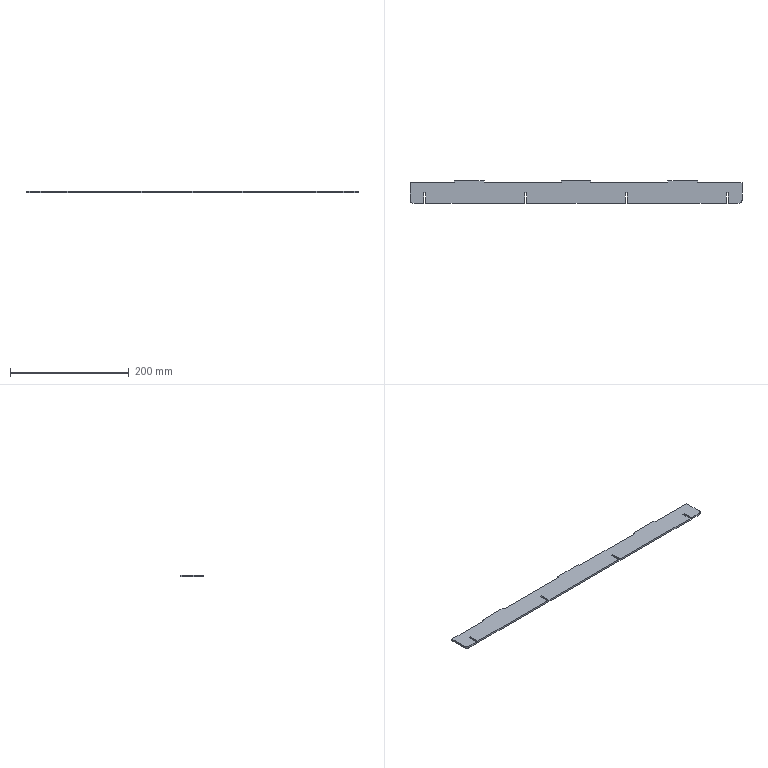Part | SolidWorks | features FlatPattern 1, SMBaseFlange 1, SheetMetal 1 | 1 solid | 36 faces | box 560 x 38 x 3.2 mm | volume 63405 mm3 | plane 34 | cylinder 2 | commonest cylinder face diameters 10 x2
STEP:
#1=CARTESIAN_POINT('',(-210.978,-661.7,0.));
#2=VERTEX_POINT('',#1);
#3=CARTESIAN_POINT('',(-285.978,-661.7,0.));
#4=VERTEX_POINT('',#3);
#5=CARTESIAN_POINT('',(-210.978,-661.7,0.));
#6=DIRECTION('',(-1.,0.,0.));
#7=VECTOR('',#6,1000.);
#8=LINE('',#5,#7);
#9=EDGE_CURVE('',#2,#4,#8,.T.);
#10=ORIENTED_EDGE('',*,*,#9,.F.);
#11=CARTESIAN_POINT('',(-210.978,-661.7,-3.2));
#12=VERTEX_POINT('',#11);
#13=CARTESIAN_POINT('',(-210.978,-661.7,-3.2));
#14=DIRECTION('',(0.,0.,1.));
#15=VECTOR('',#14,1000.);
#16=LINE('',#13,#15);
#17=EDGE_CURVE('',#12,#2,#16,.T.);
#18=ORIENTED_EDGE('',*,*,#17,.F.);
#19=CARTESIAN_POINT('',(-285.978,-661.7,-3.2));
#20=VERTEX_POINT('',#19);
#21=CARTESIAN_POINT('',(-210.978,-661.7,-3.2));
#22=DIRECTION('',(-1.,0.,0.));
#23=VECTOR('',#22,1000.);
#24=LINE('',#21,#23);
#25=EDGE_CURVE('',#12,#20,#24,.T.);
#26=ORIENTED_EDGE('',*,*,#25,.T.);
#27=CARTESIAN_POINT('',(-285.978,-661.7,-3.2));
#28=DIRECTION('',(0.,0.,1.));
#29=VECTOR('',#28,1000.);
#30=LINE('',#27,#29);
#31=EDGE_CURVE('',#20,#4,#30,.T.);
#32=ORIENTED_EDGE('',*,*,#31,.T.);
#33=EDGE_LOOP('',(#10,#18,#26,#32));
#34=FACE_OUTER_BOUND('',#33,.T.);
#35=CARTESIAN_POINT('',(-210.978,-661.7,-3.2));
#36=DIRECTION('',(0.,1.,0.));
#37=DIRECTION('',(0.,0.,1.));
#38=AXIS2_PLACEMENT_3D('',#35,#36,#37);
#39=PLANE('',#38);
#40=ADVANCED_FACE('',(#34),#39,.T.);
#41=CARTESIAN_POINT('',(-210.978,-658.7,0.));
#42=VERTEX_POINT('',#41);
#43=CARTESIAN_POINT('',(-210.978,-661.7,0.));
#44=DIRECTION('',(0.,-1.,0.));
#45=VECTOR('',#44,1000.);
#46=LINE('',#43,#45);
#47=EDGE_CURVE('',#42,#2,#46,.T.);
#48=ORIENTED_EDGE('',*,*,#47,.F.);
#49=CARTESIAN_POINT('',(-210.978,-658.7,-3.2));
#50=VERTEX_POINT('',#49);
#51=CARTESIAN_POINT('',(-210.978,-658.7,-3.2));
#52=DIRECTION('',(0.,0.,1.));
#53=VECTOR('',#52,1000.);
#54=LINE('',#51,#53);
#55=EDGE_CURVE('',#50,#42,#54,.T.);
#56=ORIENTED_EDGE('',*,*,#55,.F.);
#57=CARTESIAN_POINT('',(-210.978,-661.7,-3.2));
#58=DIRECTION('',(0.,-1.,0.));
#59=VECTOR('',#58,1000.);
#60=LINE('',#57,#59);
#61=EDGE_CURVE('',#50,#12,#60,.T.);
#62=ORIENTED_EDGE('',*,*,#61,.T.);
#63=ORIENTED_EDGE('',*,*,#17,.T.);
#64=EDGE_LOOP('',(#48,#56,#62,#63));
#65=FACE_OUTER_BOUND('',#64,.T.);
#66=CARTESIAN_POINT('',(-210.978,-661.7,-3.2));
#67=DIRECTION('',(-1.,0.,0.));
#68=DIRECTION('',(0.,0.,1.));
#69=AXIS2_PLACEMENT_3D('',#66,#67,#68);
#70=PLANE('',#69);
#71=ADVANCED_FACE('',(#65),#70,.T.);
#72=CARTESIAN_POINT('',(-160.978,-658.7,0.));
#73=VERTEX_POINT('',#72);
#74=CARTESIAN_POINT('',(-210.978,-658.7,0.));
#75=DIRECTION('',(-1.,0.,0.));
#76=VECTOR('',#75,1000.);
#77=LINE('',#74,#76);
#78=EDGE_CURVE('',#73,#42,#77,.T.);
#79=ORIENTED_EDGE('',*,*,#78,.F.);
#80=CARTESIAN_POINT('',(-160.978,-658.7,-3.2));
#81=VERTEX_POINT('',#80);
#82=CARTESIAN_POINT('',(-160.978,-658.7,-3.2));
#83=DIRECTION('',(0.,0.,1.));
#84=VECTOR('',#83,1000.);
#85=LINE('',#82,#84);
#86=EDGE_CURVE('',#81,#73,#85,.T.);
#87=ORIENTED_EDGE('',*,*,#86,.F.);
#88=CARTESIAN_POINT('',(-210.978,-658.7,-3.2));
#89=DIRECTION('',(-1.,0.,0.));
#90=VECTOR('',#89,1000.);
#91=LINE('',#88,#90);
#92=EDGE_CURVE('',#81,#50,#91,.T.);
#93=ORIENTED_EDGE('',*,*,#92,.T.);
#94=ORIENTED_EDGE('',*,*,#55,.T.);
#95=EDGE_LOOP('',(#79,#87,#93,#94));
#96=FACE_OUTER_BOUND('',#95,.T.);
#97=CARTESIAN_POINT('',(-210.978,-658.7,-3.2));
#98=DIRECTION('',(0.,1.,0.));
#99=DIRECTION('',(0.,0.,1.));
#100=AXIS2_PLACEMENT_3D('',#97,#98,#99);
#101=PLANE('',#100);
#102=ADVANCED_FACE('',(#96),#101,.T.);
#103=CARTESIAN_POINT('',(-160.978,-661.7,0.));
#104=VERTEX_POINT('',#103);
#105=CARTESIAN_POINT('',(-160.978,-658.7,0.));
#106=DIRECTION('',(0.,1.,0.));
#107=VECTOR('',#106,1000.);
#108=LINE('',#105,#107);
#109=EDGE_CURVE('',#104,#73,#108,.T.);
#110=ORIENTED_EDGE('',*,*,#109,.F.);
#111=CARTESIAN_POINT('',(-160.978,-661.7,-3.2));
#112=VERTEX_POINT('',#111);
#113=CARTESIAN_POINT('',(-160.978,-661.7,-3.2));
#114=DIRECTION('',(0.,0.,1.));
#115=VECTOR('',#114,1000.);
#116=LINE('',#113,#115);
#117=EDGE_CURVE('',#112,#104,#116,.T.);
#118=ORIENTED_EDGE('',*,*,#117,.F.);
#119=CARTESIAN_POINT('',(-160.978,-658.7,-3.2));
#120=DIRECTION('',(0.,1.,0.));
#121=VECTOR('',#120,1000.);
#122=LINE('',#119,#121);
#123=EDGE_CURVE('',#112,#81,#122,.T.);
#124=ORIENTED_EDGE('',*,*,#123,.T.);
#125=ORIENTED_EDGE('',*,*,#86,.T.);
#126=EDGE_LOOP('',(#110,#118,#124,#125));
#127=FACE_OUTER_BOUND('',#126,.T.);
#128=CARTESIAN_POINT('',(-160.978,-658.7,-3.2));
#129=DIRECTION('',(1.,0.,0.));
#130=DIRECTION('',(0.,0.,-1.));
#131=AXIS2_PLACEMENT_3D('',#128,#129,#130);
#132=PLANE('',#131);
#133=ADVANCED_FACE('',(#127),#132,.T.);
#134=CARTESIAN_POINT('',(-30.978,-661.7,0.));
#135=VERTEX_POINT('',#134);
#136=CARTESIAN_POINT('',(-160.978,-661.7,0.));
#137=DIRECTION('',(-1.,0.,0.));
#138=VECTOR('',#137,1000.);
#139=LINE('',#136,#138);
#140=EDGE_CURVE('',#135,#104,#139,.T.);
#141=ORIENTED_EDGE('',*,*,#140,.F.);
#142=CARTESIAN_POINT('',(-30.978,-661.7,-3.2));
#143=VERTEX_POINT('',#142);
#144=CARTESIAN_POINT('',(-30.978,-661.7,-3.2));
#145=DIRECTION('',(0.,0.,1.));
#146=VECTOR('',#145,1000.);
#147=LINE('',#144,#146);
#148=EDGE_CURVE('',#143,#135,#147,.T.);
#149=ORIENTED_EDGE('',*,*,#148,.F.);
#150=CARTESIAN_POINT('',(-160.978,-661.7,-3.2));
#151=DIRECTION('',(-1.,0.,0.));
#152=VECTOR('',#151,1000.);
#153=LINE('',#150,#152);
#154=EDGE_CURVE('',#143,#112,#153,.T.);
#155=ORIENTED_EDGE('',*,*,#154,.T.);
#156=ORIENTED_EDGE('',*,*,#117,.T.);
#157=EDGE_LOOP('',(#141,#149,#155,#156));
#158=FACE_OUTER_BOUND('',#157,.T.);
#159=CARTESIAN_POINT('',(-160.978,-661.7,-3.2));
#160=DIRECTION('',(0.,1.,0.));
#161=DIRECTION('',(0.,0.,1.));
#162=AXIS2_PLACEMENT_3D('',#159,#160,#161);
#163=PLANE('',#162);
#164=ADVANCED_FACE('',(#158),#163,.T.);
#165=CARTESIAN_POINT('',(-30.978,-658.7,0.));
#166=VERTEX_POINT('',#165);
#167=CARTESIAN_POINT('',(-30.978,-661.7,0.));
#168=DIRECTION('',(0.,-1.,0.));
#169=VECTOR('',#168,1000.);
#170=LINE('',#167,#169);
#171=EDGE_CURVE('',#166,#135,#170,.T.);
#172=ORIENTED_EDGE('',*,*,#171,.F.);
#173=CARTESIAN_POINT('',(-30.978,-658.7,-3.2));
#174=VERTEX_POINT('',#173);
#175=CARTESIAN_POINT('',(-30.978,-658.7,-3.2));
#176=DIRECTION('',(0.,0.,1.));
#177=VECTOR('',#176,1000.);
#178=LINE('',#175,#177);
#179=EDGE_CURVE('',#174,#166,#178,.T.);
#180=ORIENTED_EDGE('',*,*,#179,.F.);
#181=CARTESIAN_POINT('',(-30.978,-661.7,-3.2));
#182=DIRECTION('',(0.,-1.,0.));
#183=VECTOR('',#182,1000.);
#184=LINE('',#181,#183);
#185=EDGE_CURVE('',#174,#143,#184,.T.);
#186=ORIENTED_EDGE('',*,*,#185,.T.);
#187=ORIENTED_EDGE('',*,*,#148,.T.);
#188=EDGE_LOOP('',(#172,#180,#186,#187));
#189=FACE_OUTER_BOUND('',#188,.T.);
#190=CARTESIAN_POINT('',(-30.978,-661.7,-3.2));
#191=DIRECTION('',(-1.,0.,0.));
#192=DIRECTION('',(0.,-1.,0.));
#193=AXIS2_PLACEMENT_3D('',#190,#191,#192);
#194=PLANE('',#193);
#195=ADVANCED_FACE('',(#189),#194,.T.);
#196=CARTESIAN_POINT('',(19.022,-658.7,0.));
#197=VERTEX_POINT('',#196);
#198=CARTESIAN_POINT('',(-30.978,-658.7,0.));
#199=DIRECTION('',(-1.,0.,0.));
#200=VECTOR('',#199,1000.);
#201=LINE('',#198,#200);
#202=EDGE_CURVE('',#197,#166,#201,.T.);
#203=ORIENTED_EDGE('',*,*,#202,.F.);
#204=CARTESIAN_POINT('',(19.022,-658.7,-3.2));
#205=VERTEX_POINT('',#204);
#206=CARTESIAN_POINT('',(19.022,-658.7,-3.2));
#207=DIRECTION('',(0.,0.,1.));
#208=VECTOR('',#207,1000.);
#209=LINE('',#206,#208);
#210=EDGE_CURVE('',#205,#197,#209,.T.);
#211=ORIENTED_EDGE('',*,*,#210,.F.);
#212=CARTESIAN_POINT('',(-30.978,-658.7,-3.2));
#213=DIRECTION('',(-1.,0.,0.));
#214=VECTOR('',#213,1000.);
#215=LINE('',#212,#214);
#216=EDGE_CURVE('',#205,#174,#215,.T.);
#217=ORIENTED_EDGE('',*,*,#216,.T.);
#218=ORIENTED_EDGE('',*,*,#179,.T.);
#219=EDGE_LOOP('',(#203,#211,#217,#218));
#220=FACE_OUTER_BOUND('',#219,.T.);
#221=CARTESIAN_POINT('',(-30.978,-658.7,-3.2));
#222=DIRECTION('',(0.,1.,0.));
#223=DIRECTION('',(0.,0.,1.));
#224=AXIS2_PLACEMENT_3D('',#221,#222,#223);
#225=PLANE('',#224);
#226=ADVANCED_FACE('',(#220),#225,.T.);
#227=CARTESIAN_POINT('',(19.022,-661.7,0.));
#228=VERTEX_POINT('',#227);
#229=CARTESIAN_POINT('',(19.022,-658.7,0.));
#230=DIRECTION('',(0.,1.,0.));
#231=VECTOR('',#230,1000.);
#232=LINE('',#229,#231);
#233=EDGE_CURVE('',#228,#197,#232,.T.);
#234=ORIENTED_EDGE('',*,*,#233,.F.);
#235=CARTESIAN_POINT('',(19.022,-661.7,-3.2));
#236=VERTEX_POINT('',#235);
#237=CARTESIAN_POINT('',(19.022,-661.7,-3.2));
#238=DIRECTION('',(0.,0.,1.));
#239=VECTOR('',#238,1000.);
#240=LINE('',#237,#239);
#241=EDGE_CURVE('',#236,#228,#240,.T.);
#242=ORIENTED_EDGE('',*,*,#241,.F.);
#243=CARTESIAN_POINT('',(19.022,-658.7,-3.2));
#244=DIRECTION('',(0.,1.,0.));
#245=VECTOR('',#244,1000.);
#246=LINE('',#243,#245);
#247=EDGE_CURVE('',#236,#205,#246,.T.);
#248=ORIENTED_EDGE('',*,*,#247,.T.);
#249=ORIENTED_EDGE('',*,*,#210,.T.);
#250=EDGE_LOOP('',(#234,#242,#248,#249));
#251=FACE_OUTER_BOUND('',#250,.T.);
#252=CARTESIAN_POINT('',(19.022,-658.7,-3.2));
#253=DIRECTION('',(1.,0.,0.));
#254=DIRECTION('',(0.,1.,0.));
#255=AXIS2_PLACEMENT_3D('',#252,#253,#254);
#256=PLANE('',#255);
#257=ADVANCED_FACE('',(#251),#256,.T.);
#258=CARTESIAN_POINT('',(149.022,-661.7,0.));
#259=VERTEX_POINT('',#258);
#260=CARTESIAN_POINT('',(19.022,-661.7,0.));
#261=DIRECTION('',(-1.,0.,0.));
#262=VECTOR('',#261,1000.);
#263=LINE('',#260,#262);
#264=EDGE_CURVE('',#259,#228,#263,.T.);
#265=ORIENTED_EDGE('',*,*,#264,.F.);
#266=CARTESIAN_POINT('',(149.022,-661.7,-3.2));
#267=VERTEX_POINT('',#266);
#268=CARTESIAN_POINT('',(149.022,-661.7,-3.2));
#269=DIRECTION('',(0.,0.,1.));
#270=VECTOR('',#269,1000.);
#271=LINE('',#268,#270);
#272=EDGE_CURVE('',#267,#259,#271,.T.);
#273=ORIENTED_EDGE('',*,*,#272,.F.);
#274=CARTESIAN_POINT('',(19.022,-661.7,-3.2));
#275=DIRECTION('',(-1.,0.,0.));
#276=VECTOR('',#275,1000.);
#277=LINE('',#274,#276);
#278=EDGE_CURVE('',#267,#236,#277,.T.);
#279=ORIENTED_EDGE('',*,*,#278,.T.);
#280=ORIENTED_EDGE('',*,*,#241,.T.);
#281=EDGE_LOOP('',(#265,#273,#279,#280));
#282=FACE_OUTER_BOUND('',#281,.T.);
#283=CARTESIAN_POINT('',(19.022,-661.7,-3.2));
#284=DIRECTION('',(0.,1.,0.));
#285=DIRECTION('',(0.,0.,1.));
#286=AXIS2_PLACEMENT_3D('',#283,#284,#285);
#287=PLANE('',#286);
#288=ADVANCED_FACE('',(#282),#287,.T.);
#289=CARTESIAN_POINT('',(149.022,-658.7,0.));
#290=VERTEX_POINT('',#289);
#291=CARTESIAN_POINT('',(149.022,-658.7,0.));
#292=DIRECTION('',(0.,-1.,0.));
#293=VECTOR('',#292,1000.);
#294=LINE('',#291,#293);
#295=EDGE_CURVE('',#290,#259,#294,.T.);
#296=ORIENTED_EDGE('',*,*,#295,.F.);
#297=CARTESIAN_POINT('',(149.022,-658.7,-3.2));
#298=VERTEX_POINT('',#297);
#299=CARTESIAN_POINT('',(149.022,-658.7,-3.2));
#300=DIRECTION('',(0.,0.,1.));
#301=VECTOR('',#300,1000.);
#302=LINE('',#299,#301);
#303=EDGE_CURVE('',#298,#290,#302,.T.);
#304=ORIENTED_EDGE('',*,*,#303,.F.);
#305=CARTESIAN_POINT('',(149.022,-658.7,-3.2));
#306=DIRECTION('',(0.,-1.,0.));
#307=VECTOR('',#306,1000.);
#308=LINE('',#305,#307);
#309=EDGE_CURVE('',#298,#267,#308,.T.);
#310=ORIENTED_EDGE('',*,*,#309,.T.);
#311=ORIENTED_EDGE('',*,*,#272,.T.);
#312=EDGE_LOOP('',(#296,#304,#310,#311));
#313=FACE_OUTER_BOUND('',#312,.T.);
#314=CARTESIAN_POINT('',(149.022,-658.7,-3.2));
#315=DIRECTION('',(-1.,0.,0.));
#316=DIRECTION('',(0.,0.,1.));
#317=AXIS2_PLACEMENT_3D('',#314,#315,#316);
#318=PLANE('',#317);
#319=ADVANCED_FACE('',(#313),#318,.T.);
#320=CARTESIAN_POINT('',(199.022,-658.7,0.));
#321=VERTEX_POINT('',#320);
#322=CARTESIAN_POINT('',(199.022,-658.7,0.));
#323=DIRECTION('',(-1.,0.,0.));
#324=VECTOR('',#323,1000.);
#325=LINE('',#322,#324);
#326=EDGE_CURVE('',#321,#290,#325,.T.);
#327=ORIENTED_EDGE('',*,*,#326,.F.);
#328=CARTESIAN_POINT('',(199.022,-658.7,-3.2));
#329=VERTEX_POINT('',#328);
#330=CARTESIAN_POINT('',(199.022,-658.7,-3.2));
#331=DIRECTION('',(0.,0.,1.));
#332=VECTOR('',#331,1000.);
#333=LINE('',#330,#332);
#334=EDGE_CURVE('',#329,#321,#333,.T.);
#335=ORIENTED_EDGE('',*,*,#334,.F.);
#336=CARTESIAN_POINT('',(199.022,-658.7,-3.2));
#337=DIRECTION('',(-1.,0.,0.));
#338=VECTOR('',#337,1000.);
#339=LINE('',#336,#338);
#340=EDGE_CURVE('',#329,#298,#339,.T.);
#341=ORIENTED_EDGE('',*,*,#340,.T.);
#342=ORIENTED_EDGE('',*,*,#303,.T.);
#343=EDGE_LOOP('',(#327,#335,#341,#342));
#344=FACE_OUTER_BOUND('',#343,.T.);
#345=CARTESIAN_POINT('',(199.022,-658.7,-3.2));
#346=DIRECTION('',(0.,1.,0.));
#347=DIRECTION('',(0.,0.,1.));
#348=AXIS2_PLACEMENT_3D('',#345,#346,#347);
#349=PLANE('',#348);
#350=ADVANCED_FACE('',(#344),#349,.T.);
#351=CARTESIAN_POINT('',(199.022,-661.7,0.));
#352=VERTEX_POINT('',#351);
#353=CARTESIAN_POINT('',(199.022,-661.7,0.));
#354=DIRECTION('',(0.,1.,0.));
#355=VECTOR('',#354,1000.);
#356=LINE('',#353,#355);
#357=EDGE_CURVE('',#352,#321,#356,.T.);
#358=ORIENTED_EDGE('',*,*,#357,.F.);
#359=CARTESIAN_POINT('',(199.022,-661.7,-3.2));
#360=VERTEX_POINT('',#359);
#361=CARTESIAN_POINT('',(199.022,-661.7,-3.2));
#362=DIRECTION('',(0.,0.,1.));
#363=VECTOR('',#362,1000.);
#364=LINE('',#361,#363);
#365=EDGE_CURVE('',#360,#352,#364,.T.);
#366=ORIENTED_EDGE('',*,*,#365,.F.);
#367=CARTESIAN_POINT('',(199.022,-661.7,-3.2));
#368=DIRECTION('',(0.,1.,0.));
#369=VECTOR('',#368,1000.);
#370=LINE('',#367,#369);
#371=EDGE_CURVE('',#360,#329,#370,.T.);
#372=ORIENTED_EDGE('',*,*,#371,.T.);
#373=ORIENTED_EDGE('',*,*,#334,.T.);
#374=EDGE_LOOP('',(#358,#366,#372,#373));
#375=FACE_OUTER_BOUND('',#374,.T.);
#376=CARTESIAN_POINT('',(199.022,-661.7,-3.2));
#377=DIRECTION('',(1.,0.,0.));
#378=DIRECTION('',(0.,0.,-1.));
#379=AXIS2_PLACEMENT_3D('',#376,#377,#378);
#380=PLANE('',#379);
#381=ADVANCED_FACE('',(#375),#380,.T.);
#382=CARTESIAN_POINT('',(274.022,-661.7,0.));
#383=VERTEX_POINT('',#382);
#384=CARTESIAN_POINT('',(199.022,-661.7,0.));
#385=DIRECTION('',(-1.,0.,0.));
#386=VECTOR('',#385,1000.);
#387=LINE('',#384,#386);
#388=EDGE_CURVE('',#383,#352,#387,.T.);
#389=ORIENTED_EDGE('',*,*,#388,.F.);
#390=CARTESIAN_POINT('',(274.022,-661.7,-3.2));
#391=VERTEX_POINT('',#390);
#392=CARTESIAN_POINT('',(274.022,-661.7,-3.2));
#393=DIRECTION('',(0.,0.,1.));
#394=VECTOR('',#393,1000.);
#395=LINE('',#392,#394);
#396=EDGE_CURVE('',#391,#383,#395,.T.);
#397=ORIENTED_EDGE('',*,*,#396,.F.);
#398=CARTESIAN_POINT('',(199.022,-661.7,-3.2));
#399=DIRECTION('',(-1.,0.,0.));
#400=VECTOR('',#399,1000.);
#401=LINE('',#398,#400);
#402=EDGE_CURVE('',#391,#360,#401,.T.);
#403=ORIENTED_EDGE('',*,*,#402,.T.);
#404=ORIENTED_EDGE('',*,*,#365,.T.);
#405=EDGE_LOOP('',(#389,#397,#403,#404));
#406=FACE_OUTER_BOUND('',#405,.T.);
#407=CARTESIAN_POINT('',(199.022,-661.7,-3.2));
#408=DIRECTION('',(0.,1.,0.));
#409=DIRECTION('',(0.,0.,1.));
#410=AXIS2_PLACEMENT_3D('',#407,#408,#409);
#411=PLANE('',#410);
#412=ADVANCED_FACE('',(#406),#411,.T.);
#413=CARTESIAN_POINT('',(274.022,-691.7,0.));
#414=VERTEX_POINT('',#413);
#415=CARTESIAN_POINT('',(274.022,-661.7,0.));
#416=DIRECTION('',(0.,1.,0.));
#417=VECTOR('',#416,1000.);
#418=LINE('',#415,#417);
#419=EDGE_CURVE('',#414,#383,#418,.T.);
#420=ORIENTED_EDGE('',*,*,#419,.F.);
#421=CARTESIAN_POINT('',(274.022,-691.7,-3.2));
#422=VERTEX_POINT('',#421);
#423=CARTESIAN_POINT('',(274.022,-691.7,-3.2));
#424=DIRECTION('',(0.,0.,1.));
#425=VECTOR('',#424,1000.);
#426=LINE('',#423,#425);
#427=EDGE_CURVE('',#422,#414,#426,.T.);
#428=ORIENTED_EDGE('',*,*,#427,.F.);
#429=CARTESIAN_POINT('',(274.022,-661.7,-3.2));
#430=DIRECTION('',(0.,1.,0.));
#431=VECTOR('',#430,1000.);
#432=LINE('',#429,#431);
#433=EDGE_CURVE('',#422,#391,#432,.T.);
#434=ORIENTED_EDGE('',*,*,#433,.T.);
#435=ORIENTED_EDGE('',*,*,#396,.T.);
#436=EDGE_LOOP('',(#420,#428,#434,#435));
#437=FACE_OUTER_BOUND('',#436,.T.);
#438=CARTESIAN_POINT('',(274.022,-661.7,-3.2));
#439=DIRECTION('',(1.,0.,0.));
#440=DIRECTION('',(0.,0.,-1.));
#441=AXIS2_PLACEMENT_3D('',#438,#439,#440);
#442=PLANE('',#441);
#443=ADVANCED_FACE('',(#437),#442,.T.);
#444=CARTESIAN_POINT('',(269.022,-696.7,0.));
#445=VERTEX_POINT('',#444);
#446=CARTESIAN_POINT('',(269.022,-691.7,0.));
#447=DIRECTION('',(0.,0.,1.));
#448=DIRECTION('',(1.,0.,0.));
#449=AXIS2_PLACEMENT_3D('',#446,#447,#448);
#450=CIRCLE('',#449,5.);
#451=EDGE_CURVE('',#445,#414,#450,.T.);
#452=ORIENTED_EDGE('',*,*,#451,.F.);
#453=CARTESIAN_POINT('',(269.022,-696.7,-3.2));
#454=VERTEX_POINT('',#453);
#455=CARTESIAN_POINT('',(269.022,-696.7,-3.2));
#456=DIRECTION('',(0.,0.,1.));
#457=VECTOR('',#456,1000.);
#458=LINE('',#455,#457);
#459=EDGE_CURVE('',#454,#445,#458,.T.);
#460=ORIENTED_EDGE('',*,*,#459,.F.);
#461=CARTESIAN_POINT('',(269.022,-691.7,-3.2));
#462=DIRECTION('',(0.,0.,1.));
#463=DIRECTION('',(1.,0.,0.));
#464=AXIS2_PLACEMENT_3D('',#461,#462,#463);
#465=CIRCLE('',#464,5.);
#466=EDGE_CURVE('',#454,#422,#465,.T.);
#467=ORIENTED_EDGE('',*,*,#466,.T.);
#468=ORIENTED_EDGE('',*,*,#427,.T.);
#469=EDGE_LOOP('',(#452,#460,#467,#468));
#470=FACE_OUTER_BOUND('',#469,.T.);
#471=CARTESIAN_POINT('',(269.022,-691.7,-3.2));
#472=DIRECTION('',(0.,0.,1.));
#473=DIRECTION('',(1.,0.,0.));
#474=AXIS2_PLACEMENT_3D('',#471,#472,#473);
#475=CYLINDRICAL_SURFACE('',#474,5.);
#476=ADVANCED_FACE('',(#470),#475,.T.);
#477=CARTESIAN_POINT('',(250.622,-696.7,0.));
#478=VERTEX_POINT('',#477);
#479=CARTESIAN_POINT('',(250.622,-696.7,0.));
#480=DIRECTION('',(1.,0.,0.));
#481=VECTOR('',#480,1000.);
#482=LINE('',#479,#481);
#483=EDGE_CURVE('',#478,#445,#482,.T.);
#484=ORIENTED_EDGE('',*,*,#483,.F.);
#485=CARTESIAN_POINT('',(250.622,-696.7,-3.2));
#486=VERTEX_POINT('',#485);
#487=CARTESIAN_POINT('',(250.622,-696.7,-3.2));
#488=DIRECTION('',(0.,0.,1.));
#489=VECTOR('',#488,1000.);
#490=LINE('',#487,#489);
#491=EDGE_CURVE('',#486,#478,#490,.T.);
#492=ORIENTED_EDGE('',*,*,#491,.F.);
#493=CARTESIAN_POINT('',(250.622,-696.7,-3.2));
#494=DIRECTION('',(1.,0.,0.));
#495=VECTOR('',#494,1000.);
#496=LINE('',#493,#495);
#497=EDGE_CURVE('',#486,#454,#496,.T.);
#498=ORIENTED_EDGE('',*,*,#497,.T.);
#499=ORIENTED_EDGE('',*,*,#459,.T.);
#500=EDGE_LOOP('',(#484,#492,#498,#499));
#501=FACE_OUTER_BOUND('',#500,.T.);
#502=CARTESIAN_POINT('',(250.622,-696.7,-3.2));
#503=DIRECTION('',(0.,-1.,0.));
#504=DIRECTION('',(0.,0.,-1.));
#505=AXIS2_PLACEMENT_3D('',#502,#503,#504);
#506=PLANE('',#505);
#507=ADVANCED_FACE('',(#501),#506,.T.);
#508=CARTESIAN_POINT('',(250.622,-679.1,0.));
#509=VERTEX_POINT('',#508);
#510=CARTESIAN_POINT('',(250.622,-679.1,0.));
#511=DIRECTION('',(0.,-1.,0.));
#512=VECTOR('',#511,1000.);
#513=LINE('',#510,#512);
#514=EDGE_CURVE('',#509,#478,#513,.T.);
#515=ORIENTED_EDGE('',*,*,#514,.F.);
#516=CARTESIAN_POINT('',(250.622,-679.1,-3.2));
#517=VERTEX_POINT('',#516);
#518=CARTESIAN_POINT('',(250.622,-679.1,-3.2));
#519=DIRECTION('',(0.,0.,1.));
#520=VECTOR('',#519,1000.);
#521=LINE('',#518,#520);
#522=EDGE_CURVE('',#517,#509,#521,.T.);
#523=ORIENTED_EDGE('',*,*,#522,.F.);
#524=CARTESIAN_POINT('',(250.622,-679.1,-3.2));
#525=DIRECTION('',(0.,-1.,0.));
#526=VECTOR('',#525,1000.);
#527=LINE('',#524,#526);
#528=EDGE_CURVE('',#517,#486,#527,.T.);
#529=ORIENTED_EDGE('',*,*,#528,.T.);
#530=ORIENTED_EDGE('',*,*,#491,.T.);
#531=EDGE_LOOP('',(#515,#523,#529,#530));
#532=FACE_OUTER_BOUND('',#531,.T.);
#533=CARTESIAN_POINT('',(250.622,-679.1,-3.2));
#534=DIRECTION('',(-1.,0.,0.));
#535=DIRECTION('',(0.,0.,1.));
#536=AXIS2_PLACEMENT_3D('',#533,#534,#535);
#537=PLANE('',#536);
#538=ADVANCED_FACE('',(#532),#537,.T.);
#539=CARTESIAN_POINT('',(247.422,-679.1,0.));
#540=VERTEX_POINT('',#539);
#541=CARTESIAN_POINT('',(247.422,-679.1,0.));
#542=DIRECTION('',(1.,0.,0.));
#543=VECTOR('',#542,1000.);
#544=LINE('',#541,#543);
#545=EDGE_CURVE('',#540,#509,#544,.T.);
#546=ORIENTED_EDGE('',*,*,#545,.F.);
#547=CARTESIAN_POINT('',(247.422,-679.1,-3.2));
#548=VERTEX_POINT('',#547);
#549=CARTESIAN_POINT('',(247.422,-679.1,-3.2));
#550=DIRECTION('',(0.,0.,1.));
#551=VECTOR('',#550,1000.);
#552=LINE('',#549,#551);
#553=EDGE_CURVE('',#548,#540,#552,.T.);
#554=ORIENTED_EDGE('',*,*,#553,.F.);
#555=CARTESIAN_POINT('',(247.422,-679.1,-3.2));
#556=DIRECTION('',(1.,0.,0.));
#557=VECTOR('',#556,1000.);
#558=LINE('',#555,#557);
#559=EDGE_CURVE('',#548,#517,#558,.T.);
#560=ORIENTED_EDGE('',*,*,#559,.T.);
#561=ORIENTED_EDGE('',*,*,#522,.T.);
#562=EDGE_LOOP('',(#546,#554,#560,#561));
#563=FACE_OUTER_BOUND('',#562,.T.);
#564=CARTESIAN_POINT('',(247.422,-679.1,-3.2));
#565=DIRECTION('',(0.,-1.,0.));
#566=DIRECTION('',(0.,0.,-1.));
#567=AXIS2_PLACEMENT_3D('',#564,#565,#566);
#568=PLANE('',#567);
#569=ADVANCED_FACE('',(#563),#568,.T.);
#570=CARTESIAN_POINT('',(247.422,-696.7,0.));
#571=VERTEX_POINT('',#570);
#572=CARTESIAN_POINT('',(247.422,-696.7,0.));
#573=DIRECTION('',(0.,1.,0.));
#574=VECTOR('',#573,1000.);
#575=LINE('',#572,#574);
#576=EDGE_CURVE('',#571,#540,#575,.T.);
#577=ORIENTED_EDGE('',*,*,#576,.F.);
#578=CARTESIAN_POINT('',(247.422,-696.7,-3.2));
#579=VERTEX_POINT('',#578);
#580=CARTESIAN_POINT('',(247.422,-696.7,-3.2));
#581=DIRECTION('',(0.,0.,1.));
#582=VECTOR('',#581,1000.);
#583=LINE('',#580,#582);
#584=EDGE_CURVE('',#579,#571,#583,.T.);
#585=ORIENTED_EDGE('',*,*,#584,.F.);
#586=CARTESIAN_POINT('',(247.422,-696.7,-3.2));
#587=DIRECTION('',(0.,1.,0.));
#588=VECTOR('',#587,1000.);
#589=LINE('',#586,#588);
#590=EDGE_CURVE('',#579,#548,#589,.T.);
#591=ORIENTED_EDGE('',*,*,#590,.T.);
#592=ORIENTED_EDGE('',*,*,#553,.T.);
#593=EDGE_LOOP('',(#577,#585,#591,#592));
#594=FACE_OUTER_BOUND('',#593,.T.);
#595=CARTESIAN_POINT('',(247.422,-696.7,-3.2));
#596=DIRECTION('',(1.,0.,0.));
#597=DIRECTION('',(0.,0.,-1.));
#598=AXIS2_PLACEMENT_3D('',#595,#596,#597);
#599=PLANE('',#598);
#600=ADVANCED_FACE('',(#594),#599,.T.);
#601=CARTESIAN_POINT('',(80.622,-696.7,0.));
#602=VERTEX_POINT('',#601);
#603=CARTESIAN_POINT('',(80.622,-696.7,0.));
#604=DIRECTION('',(1.,0.,0.));
#605=VECTOR('',#604,1000.);
#606=LINE('',#603,#605);
#607=EDGE_CURVE('',#602,#571,#606,.T.);
#608=ORIENTED_EDGE('',*,*,#607,.F.);
#609=CARTESIAN_POINT('',(80.622,-696.7,-3.2));
#610=VERTEX_POINT('',#609);
#611=CARTESIAN_POINT('',(80.622,-696.7,-3.2));
#612=DIRECTION('',(0.,0.,1.));
#613=VECTOR('',#612,1000.);
#614=LINE('',#611,#613);
#615=EDGE_CURVE('',#610,#602,#614,.T.);
#616=ORIENTED_EDGE('',*,*,#615,.F.);
#617=CARTESIAN_POINT('',(80.622,-696.7,-3.2));
#618=DIRECTION('',(1.,0.,0.));
#619=VECTOR('',#618,1000.);
#620=LINE('',#617,#619);
#621=EDGE_CURVE('',#610,#579,#620,.T.);
#622=ORIENTED_EDGE('',*,*,#621,.T.);
#623=ORIENTED_EDGE('',*,*,#584,.T.);
#624=EDGE_LOOP('',(#608,#616,#622,#623));
#625=FACE_OUTER_BOUND('',#624,.T.);
#626=CARTESIAN_POINT('',(80.622,-696.7,-3.2));
#627=DIRECTION('',(0.,-1.,0.));
#628=DIRECTION('',(0.,0.,-1.));
#629=AXIS2_PLACEMENT_3D('',#626,#627,#628);
#630=PLANE('',#629);
#631=ADVANCED_FACE('',(#625),#630,.T.);
#632=CARTESIAN_POINT('',(80.622,-679.1,0.));
#633=VERTEX_POINT('',#632);
#634=CARTESIAN_POINT('',(80.622,-679.1,0.));
#635=DIRECTION('',(0.,-1.,0.));
#636=VECTOR('',#635,1000.);
#637=LINE('',#634,#636);
#638=EDGE_CURVE('',#633,#602,#637,.T.);
#639=ORIENTED_EDGE('',*,*,#638,.F.);
#640=CARTESIAN_POINT('',(80.622,-679.1,-3.2));
#641=VERTEX_POINT('',#640);
#642=CARTESIAN_POINT('',(80.622,-679.1,-3.2));
#643=DIRECTION('',(0.,0.,1.));
#644=VECTOR('',#643,1000.);
#645=LINE('',#642,#644);
#646=EDGE_CURVE('',#641,#633,#645,.T.);
#647=ORIENTED_EDGE('',*,*,#646,.F.);
#648=CARTESIAN_POINT('',(80.622,-679.1,-3.2));
#649=DIRECTION('',(0.,-1.,0.));
#650=VECTOR('',#649,1000.);
#651=LINE('',#648,#650);
#652=EDGE_CURVE('',#641,#610,#651,.T.);
#653=ORIENTED_EDGE('',*,*,#652,.T.);
#654=ORIENTED_EDGE('',*,*,#615,.T.);
#655=EDGE_LOOP('',(#639,#647,#653,#654));
#656=FACE_OUTER_BOUND('',#655,.T.);
#657=CARTESIAN_POINT('',(80.622,-679.1,-3.2));
#658=DIRECTION('',(-1.,0.,0.));
#659=DIRECTION('',(0.,0.,1.));
#660=AXIS2_PLACEMENT_3D('',#657,#658,#659);
#661=PLANE('',#660);
#662=ADVANCED_FACE('',(#656),#661,.T.);
#663=CARTESIAN_POINT('',(77.422,-679.1,0.));
#664=VERTEX_POINT('',#663);
#665=CARTESIAN_POINT('',(77.422,-679.1,0.));
#666=DIRECTION('',(1.,0.,0.));
#667=VECTOR('',#666,1000.);
#668=LINE('',#665,#667);
#669=EDGE_CURVE('',#664,#633,#668,.T.);
#670=ORIENTED_EDGE('',*,*,#669,.F.);
#671=CARTESIAN_POINT('',(77.422,-679.1,-3.2));
#672=VERTEX_POINT('',#671);
#673=CARTESIAN_POINT('',(77.422,-679.1,-3.2));
#674=DIRECTION('',(0.,0.,1.));
#675=VECTOR('',#674,1000.);
#676=LINE('',#673,#675);
#677=EDGE_CURVE('',#672,#664,#676,.T.);
#678=ORIENTED_EDGE('',*,*,#677,.F.);
#679=CARTESIAN_POINT('',(77.422,-679.1,-3.2));
#680=DIRECTION('',(1.,0.,0.));
#681=VECTOR('',#680,1000.);
#682=LINE('',#679,#681);
#683=EDGE_CURVE('',#672,#641,#682,.T.);
#684=ORIENTED_EDGE('',*,*,#683,.T.);
#685=ORIENTED_EDGE('',*,*,#646,.T.);
#686=EDGE_LOOP('',(#670,#678,#684,#685));
#687=FACE_OUTER_BOUND('',#686,.T.);
#688=CARTESIAN_POINT('',(77.422,-679.1,-3.2));
#689=DIRECTION('',(0.,-1.,0.));
#690=DIRECTION('',(0.,0.,-1.));
#691=AXIS2_PLACEMENT_3D('',#688,#689,#690);
#692=PLANE('',#691);
#693=ADVANCED_FACE('',(#687),#692,.T.);
#694=CARTESIAN_POINT('',(77.422,-696.7,0.));
#695=VERTEX_POINT('',#694);
#696=CARTESIAN_POINT('',(77.422,-696.7,0.));
#697=DIRECTION('',(0.,1.,0.));
#698=VECTOR('',#697,1000.);
#699=LINE('',#696,#698);
#700=EDGE_CURVE('',#695,#664,#699,.T.);
#701=ORIENTED_EDGE('',*,*,#700,.F.);
#702=CARTESIAN_POINT('',(77.422,-696.7,-3.2));
#703=VERTEX_POINT('',#702);
#704=CARTESIAN_POINT('',(77.422,-696.7,-3.2));
#705=DIRECTION('',(0.,0.,1.));
#706=VECTOR('',#705,1000.);
#707=LINE('',#704,#706);
#708=EDGE_CURVE('',#703,#695,#707,.T.);
#709=ORIENTED_EDGE('',*,*,#708,.F.);
#710=CARTESIAN_POINT('',(77.422,-696.7,-3.2));
#711=DIRECTION('',(0.,1.,0.));
#712=VECTOR('',#711,1000.);
#713=LINE('',#710,#712);
#714=EDGE_CURVE('',#703,#672,#713,.T.);
#715=ORIENTED_EDGE('',*,*,#714,.T.);
#716=ORIENTED_EDGE('',*,*,#677,.T.);
#717=EDGE_LOOP('',(#701,#709,#715,#716));
#718=FACE_OUTER_BOUND('',#717,.T.);
#719=CARTESIAN_POINT('',(77.422,-696.7,-3.2));
#720=DIRECTION('',(1.,0.,0.));
#721=DIRECTION('',(0.,0.,-1.));
#722=AXIS2_PLACEMENT_3D('',#719,#720,#721);
#723=PLANE('',#722);
#724=ADVANCED_FACE('',(#718),#723,.T.);
#725=CARTESIAN_POINT('',(-89.378,-696.7,0.));
#726=VERTEX_POINT('',#725);
#727=CARTESIAN_POINT('',(-89.378,-696.7,0.));
#728=DIRECTION('',(1.,0.,0.));
#729=VECTOR('',#728,1000.);
#730=LINE('',#727,#729);
#731=EDGE_CURVE('',#726,#695,#730,.T.);
#732=ORIENTED_EDGE('',*,*,#731,.F.);
#733=CARTESIAN_POINT('',(-89.378,-696.7,-3.2));
#734=VERTEX_POINT('',#733);
#735=CARTESIAN_POINT('',(-89.378,-696.7,-3.2));
#736=DIRECTION('',(0.,0.,1.));
#737=VECTOR('',#736,1000.);
#738=LINE('',#735,#737);
#739=EDGE_CURVE('',#734,#726,#738,.T.);
#740=ORIENTED_EDGE('',*,*,#739,.F.);
#741=CARTESIAN_POINT('',(-89.378,-696.7,-3.2));
#742=DIRECTION('',(1.,0.,0.));
#743=VECTOR('',#742,1000.);
#744=LINE('',#741,#743);
#745=EDGE_CURVE('',#734,#703,#744,.T.);
#746=ORIENTED_EDGE('',*,*,#745,.T.);
#747=ORIENTED_EDGE('',*,*,#708,.T.);
#748=EDGE_LOOP('',(#732,#740,#746,#747));
#749=FACE_OUTER_BOUND('',#748,.T.);
#750=CARTESIAN_POINT('',(-89.378,-696.7,-3.2));
#751=DIRECTION('',(0.,-1.,0.));
#752=DIRECTION('',(0.,0.,-1.));
#753=AXIS2_PLACEMENT_3D('',#750,#751,#752);
#754=PLANE('',#753);
#755=ADVANCED_FACE('',(#749),#754,.T.);
#756=CARTESIAN_POINT('',(-89.378,-679.1,0.));
#757=VERTEX_POINT('',#756);
#758=CARTESIAN_POINT('',(-89.378,-679.1,0.));
#759=DIRECTION('',(0.,-1.,0.));
#760=VECTOR('',#759,1000.);
#761=LINE('',#758,#760);
#762=EDGE_CURVE('',#757,#726,#761,.T.);
#763=ORIENTED_EDGE('',*,*,#762,.F.);
#764=CARTESIAN_POINT('',(-89.378,-679.1,-3.2));
#765=VERTEX_POINT('',#764);
#766=CARTESIAN_POINT('',(-89.378,-679.1,-3.2));
#767=DIRECTION('',(0.,0.,1.));
#768=VECTOR('',#767,1000.);
#769=LINE('',#766,#768);
#770=EDGE_CURVE('',#765,#757,#769,.T.);
#771=ORIENTED_EDGE('',*,*,#770,.F.);
#772=CARTESIAN_POINT('',(-89.378,-679.1,-3.2));
#773=DIRECTION('',(0.,-1.,0.));
#774=VECTOR('',#773,1000.);
#775=LINE('',#772,#774);
#776=EDGE_CURVE('',#765,#734,#775,.T.);
#777=ORIENTED_EDGE('',*,*,#776,.T.);
#778=ORIENTED_EDGE('',*,*,#739,.T.);
#779=EDGE_LOOP('',(#763,#771,#777,#778));
#780=FACE_OUTER_BOUND('',#779,.T.);
#781=CARTESIAN_POINT('',(-89.378,-679.1,-3.2));
#782=DIRECTION('',(-1.,0.,0.));
#783=DIRECTION('',(0.,0.,1.));
#784=AXIS2_PLACEMENT_3D('',#781,#782,#783);
#785=PLANE('',#784);
#786=ADVANCED_FACE('',(#780),#785,.T.);
#787=CARTESIAN_POINT('',(-92.578,-679.1,0.));
#788=VERTEX_POINT('',#787);
#789=CARTESIAN_POINT('',(-92.578,-679.1,0.));
#790=DIRECTION('',(1.,0.,0.));
#791=VECTOR('',#790,1000.);
#792=LINE('',#789,#791);
#793=EDGE_CURVE('',#788,#757,#792,.T.);
#794=ORIENTED_EDGE('',*,*,#793,.F.);
#795=CARTESIAN_POINT('',(-92.578,-679.1,-3.2));
#796=VERTEX_POINT('',#795);
#797=CARTESIAN_POINT('',(-92.578,-679.1,-3.2));
#798=DIRECTION('',(0.,0.,1.));
#799=VECTOR('',#798,1000.);
#800=LINE('',#797,#799);
#801=EDGE_CURVE('',#796,#788,#800,.T.);
#802=ORIENTED_EDGE('',*,*,#801,.F.);
#803=CARTESIAN_POINT('',(-92.578,-679.1,-3.2));
#804=DIRECTION('',(1.,0.,0.));
#805=VECTOR('',#804,1000.);
#806=LINE('',#803,#805);
#807=EDGE_CURVE('',#796,#765,#806,.T.);
#808=ORIENTED_EDGE('',*,*,#807,.T.);
#809=ORIENTED_EDGE('',*,*,#770,.T.);
#810=EDGE_LOOP('',(#794,#802,#808,#809));
#811=FACE_OUTER_BOUND('',#810,.T.);
#812=CARTESIAN_POINT('',(-92.578,-679.1,-3.2));
#813=DIRECTION('',(0.,-1.,0.));
#814=DIRECTION('',(0.,0.,-1.));
#815=AXIS2_PLACEMENT_3D('',#812,#813,#814);
#816=PLANE('',#815);
#817=ADVANCED_FACE('',(#811),#816,.T.);
#818=CARTESIAN_POINT('',(-92.578,-696.7,0.));
#819=VERTEX_POINT('',#818);
#820=CARTESIAN_POINT('',(-92.578,-696.7,0.));
#821=DIRECTION('',(0.,1.,0.));
#822=VECTOR('',#821,1000.);
#823=LINE('',#820,#822);
#824=EDGE_CURVE('',#819,#788,#823,.T.);
#825=ORIENTED_EDGE('',*,*,#824,.F.);
#826=CARTESIAN_POINT('',(-92.578,-696.7,-3.2));
#827=VERTEX_POINT('',#826);
#828=CARTESIAN_POINT('',(-92.578,-696.7,-3.2));
#829=DIRECTION('',(0.,0.,1.));
#830=VECTOR('',#829,1000.);
#831=LINE('',#828,#830);
#832=EDGE_CURVE('',#827,#819,#831,.T.);
#833=ORIENTED_EDGE('',*,*,#832,.F.);
#834=CARTESIAN_POINT('',(-92.578,-696.7,-3.2));
#835=DIRECTION('',(0.,1.,0.));
#836=VECTOR('',#835,1000.);
#837=LINE('',#834,#836);
#838=EDGE_CURVE('',#827,#796,#837,.T.);
#839=ORIENTED_EDGE('',*,*,#838,.T.);
#840=ORIENTED_EDGE('',*,*,#801,.T.);
#841=EDGE_LOOP('',(#825,#833,#839,#840));
#842=FACE_OUTER_BOUND('',#841,.T.);
#843=CARTESIAN_POINT('',(-92.578,-696.7,-3.2));
#844=DIRECTION('',(1.,0.,0.));
#845=DIRECTION('',(0.,0.,-1.));
#846=AXIS2_PLACEMENT_3D('',#843,#844,#845);
#847=PLANE('',#846);
#848=ADVANCED_FACE('',(#842),#847,.T.);
#849=CARTESIAN_POINT('',(-259.378,-696.7,0.));
#850=VERTEX_POINT('',#849);
#851=CARTESIAN_POINT('',(-259.378,-696.7,0.));
#852=DIRECTION('',(1.,0.,0.));
#853=VECTOR('',#852,1000.);
#854=LINE('',#851,#853);
#855=EDGE_CURVE('',#850,#819,#854,.T.);
#856=ORIENTED_EDGE('',*,*,#855,.F.);
#857=CARTESIAN_POINT('',(-259.378,-696.7,-3.2));
#858=VERTEX_POINT('',#857);
#859=CARTESIAN_POINT('',(-259.378,-696.7,-3.2));
#860=DIRECTION('',(0.,0.,1.));
#861=VECTOR('',#860,1000.);
#862=LINE('',#859,#861);
#863=EDGE_CURVE('',#858,#850,#862,.T.);
#864=ORIENTED_EDGE('',*,*,#863,.F.);
#865=CARTESIAN_POINT('',(-259.378,-696.7,-3.2));
#866=DIRECTION('',(1.,0.,0.));
#867=VECTOR('',#866,1000.);
#868=LINE('',#865,#867);
#869=EDGE_CURVE('',#858,#827,#868,.T.);
#870=ORIENTED_EDGE('',*,*,#869,.T.);
#871=ORIENTED_EDGE('',*,*,#832,.T.);
#872=EDGE_LOOP('',(#856,#864,#870,#871));
#873=FACE_OUTER_BOUND('',#872,.T.);
#874=CARTESIAN_POINT('',(-259.378,-696.7,-3.2));
#875=DIRECTION('',(0.,-1.,0.));
#876=DIRECTION('',(0.,0.,-1.));
#877=AXIS2_PLACEMENT_3D('',#874,#875,#876);
#878=PLANE('',#877);
#879=ADVANCED_FACE('',(#873),#878,.T.);
#880=CARTESIAN_POINT('',(-259.378,-679.1,0.));
#881=VERTEX_POINT('',#880);
#882=CARTESIAN_POINT('',(-259.378,-679.1,0.));
#883=DIRECTION('',(0.,-1.,0.));
#884=VECTOR('',#883,1000.);
#885=LINE('',#882,#884);
#886=EDGE_CURVE('',#881,#850,#885,.T.);
#887=ORIENTED_EDGE('',*,*,#886,.F.);
#888=CARTESIAN_POINT('',(-259.378,-679.1,-3.2));
#889=VERTEX_POINT('',#888);
#890=CARTESIAN_POINT('',(-259.378,-679.1,-3.2));
#891=DIRECTION('',(0.,0.,1.));
#892=VECTOR('',#891,1000.);
#893=LINE('',#890,#892);
#894=EDGE_CURVE('',#889,#881,#893,.T.);
#895=ORIENTED_EDGE('',*,*,#894,.F.);
#896=CARTESIAN_POINT('',(-259.378,-679.1,-3.2));
#897=DIRECTION('',(0.,-1.,0.));
#898=VECTOR('',#897,1000.);
#899=LINE('',#896,#898);
#900=EDGE_CURVE('',#889,#858,#899,.T.);
#901=ORIENTED_EDGE('',*,*,#900,.T.);
#902=ORIENTED_EDGE('',*,*,#863,.T.);
#903=EDGE_LOOP('',(#887,#895,#901,#902));
#904=FACE_OUTER_BOUND('',#903,.T.);
#905=CARTESIAN_POINT('',(-259.378,-679.1,-3.2));
#906=DIRECTION('',(-1.,0.,0.));
#907=DIRECTION('',(0.,0.,1.));
#908=AXIS2_PLACEMENT_3D('',#905,#906,#907);
#909=PLANE('',#908);
#910=ADVANCED_FACE('',(#904),#909,.T.);
#911=CARTESIAN_POINT('',(-262.578,-679.1,0.));
#912=VERTEX_POINT('',#911);
#913=CARTESIAN_POINT('',(-262.578,-679.1,0.));
#914=DIRECTION('',(1.,0.,0.));
#915=VECTOR('',#914,1000.);
#916=LINE('',#913,#915);
#917=EDGE_CURVE('',#912,#881,#916,.T.);
#918=ORIENTED_EDGE('',*,*,#917,.F.);
#919=CARTESIAN_POINT('',(-262.578,-679.1,-3.2));
#920=VERTEX_POINT('',#919);
#921=CARTESIAN_POINT('',(-262.578,-679.1,-3.2));
#922=DIRECTION('',(0.,0.,1.));
#923=VECTOR('',#922,1000.);
#924=LINE('',#921,#923);
#925=EDGE_CURVE('',#920,#912,#924,.T.);
#926=ORIENTED_EDGE('',*,*,#925,.F.);
#927=CARTESIAN_POINT('',(-262.578,-679.1,-3.2));
#928=DIRECTION('',(1.,0.,0.));
#929=VECTOR('',#928,1000.);
#930=LINE('',#927,#929);
#931=EDGE_CURVE('',#920,#889,#930,.T.);
#932=ORIENTED_EDGE('',*,*,#931,.T.);
#933=ORIENTED_EDGE('',*,*,#894,.T.);
#934=EDGE_LOOP('',(#918,#926,#932,#933));
#935=FACE_OUTER_BOUND('',#934,.T.);
#936=CARTESIAN_POINT('',(-262.578,-679.1,-3.2));
#937=DIRECTION('',(0.,-1.,0.));
#938=DIRECTION('',(0.,0.,-1.));
#939=AXIS2_PLACEMENT_3D('',#936,#937,#938);
#940=PLANE('',#939);
#941=ADVANCED_FACE('',(#935),#940,.T.);
#942=CARTESIAN_POINT('',(-262.578,-696.7,0.));
#943=VERTEX_POINT('',#942);
#944=CARTESIAN_POINT('',(-262.578,-696.7,0.));
#945=DIRECTION('',(0.,1.,0.));
#946=VECTOR('',#945,1000.);
#947=LINE('',#944,#946);
#948=EDGE_CURVE('',#943,#912,#947,.T.);
#949=ORIENTED_EDGE('',*,*,#948,.F.);
#950=CARTESIAN_POINT('',(-262.578,-696.7,-3.2));
#951=VERTEX_POINT('',#950);
#952=CARTESIAN_POINT('',(-262.578,-696.7,-3.2));
#953=DIRECTION('',(0.,0.,1.));
#954=VECTOR('',#953,1000.);
#955=LINE('',#952,#954);
#956=EDGE_CURVE('',#951,#943,#955,.T.);
#957=ORIENTED_EDGE('',*,*,#956,.F.);
#958=CARTESIAN_POINT('',(-262.578,-696.7,-3.2));
#959=DIRECTION('',(0.,1.,0.));
#960=VECTOR('',#959,1000.);
#961=LINE('',#958,#960);
#962=EDGE_CURVE('',#951,#920,#961,.T.);
#963=ORIENTED_EDGE('',*,*,#962,.T.);
#964=ORIENTED_EDGE('',*,*,#925,.T.);
#965=EDGE_LOOP('',(#949,#957,#963,#964));
#966=FACE_OUTER_BOUND('',#965,.T.);
#967=CARTESIAN_POINT('',(-262.578,-696.7,-3.2));
#968=DIRECTION('',(1.,0.,0.));
#969=DIRECTION('',(0.,0.,-1.));
#970=AXIS2_PLACEMENT_3D('',#967,#968,#969);
#971=PLANE('',#970);
#972=ADVANCED_FACE('',(#966),#971,.T.);
#973=CARTESIAN_POINT('',(-280.978,-696.7,0.));
#974=VERTEX_POINT('',#973);
#975=CARTESIAN_POINT('',(-280.978,-696.7,0.));
#976=DIRECTION('',(1.,0.,0.));
#977=VECTOR('',#976,1000.);
#978=LINE('',#975,#977);
#979=EDGE_CURVE('',#974,#943,#978,.T.);
#980=ORIENTED_EDGE('',*,*,#979,.F.);
#981=CARTESIAN_POINT('',(-280.978,-696.7,-3.2));
#982=VERTEX_POINT('',#981);
#983=CARTESIAN_POINT('',(-280.978,-696.7,-3.2));
#984=DIRECTION('',(0.,0.,1.));
#985=VECTOR('',#984,1000.);
#986=LINE('',#983,#985);
#987=EDGE_CURVE('',#982,#974,#986,.T.);
#988=ORIENTED_EDGE('',*,*,#987,.F.);
#989=CARTESIAN_POINT('',(-280.978,-696.7,-3.2));
#990=DIRECTION('',(1.,0.,0.));
#991=VECTOR('',#990,1000.);
#992=LINE('',#989,#991);
#993=EDGE_CURVE('',#982,#951,#992,.T.);
#994=ORIENTED_EDGE('',*,*,#993,.T.);
#995=ORIENTED_EDGE('',*,*,#956,.T.);
#996=EDGE_LOOP('',(#980,#988,#994,#995));
#997=FACE_OUTER_BOUND('',#996,.T.);
#998=CARTESIAN_POINT('',(-280.978,-696.7,-3.2));
#999=DIRECTION('',(0.,-1.,0.));
#1000=DIRECTION('',(0.,0.,-1.));
#1001=AXIS2_PLACEMENT_3D('',#998,#999,#1000);
#1002=PLANE('',#1001);
#1003=ADVANCED_FACE('',(#997),#1002,.T.);
#1004=CARTESIAN_POINT('',(-285.978,-691.7,0.));
#1005=VERTEX_POINT('',#1004);
#1006=CARTESIAN_POINT('',(-280.978,-691.7,0.));
#1007=DIRECTION('',(0.,0.,1.));
#1008=DIRECTION('',(1.,0.,0.));
#1009=AXIS2_PLACEMENT_3D('',#1006,#1007,#1008);
#1010=CIRCLE('',#1009,5.);
#1011=EDGE_CURVE('',#1005,#974,#1010,.T.);
#1012=ORIENTED_EDGE('',*,*,#1011,.F.);
#1013=CARTESIAN_POINT('',(-285.978,-691.7,-3.2));
#1014=VERTEX_POINT('',#1013);
#1015=CARTESIAN_POINT('',(-285.978,-691.7,-3.2));
#1016=DIRECTION('',(0.,0.,1.));
#1017=VECTOR('',#1016,1000.);
#1018=LINE('',#1015,#1017);
#1019=EDGE_CURVE('',#1014,#1005,#1018,.T.);
#1020=ORIENTED_EDGE('',*,*,#1019,.F.);
#1021=CARTESIAN_POINT('',(-280.978,-691.7,-3.2));
#1022=DIRECTION('',(0.,0.,1.));
#1023=DIRECTION('',(1.,0.,0.));
#1024=AXIS2_PLACEMENT_3D('',#1021,#1022,#1023);
#1025=CIRCLE('',#1024,5.);
#1026=EDGE_CURVE('',#1014,#982,#1025,.T.);
#1027=ORIENTED_EDGE('',*,*,#1026,.T.);
#1028=ORIENTED_EDGE('',*,*,#987,.T.);
#1029=EDGE_LOOP('',(#1012,#1020,#1027,#1028));
#1030=FACE_OUTER_BOUND('',#1029,.T.);
#1031=CARTESIAN_POINT('',(-280.978,-691.7,-3.2));
#1032=DIRECTION('',(0.,0.,1.));
#1033=DIRECTION('',(1.,0.,0.));
#1034=AXIS2_PLACEMENT_3D('',#1031,#1032,#1033);
#1035=CYLINDRICAL_SURFACE('',#1034,5.);
#1036=ADVANCED_FACE('',(#1030),#1035,.T.);
#1037=CARTESIAN_POINT('',(-285.978,-661.7,0.));
#1038=DIRECTION('',(0.,-1.,0.));
#1039=VECTOR('',#1038,1000.);
#1040=LINE('',#1037,#1039);
#1041=EDGE_CURVE('',#4,#1005,#1040,.T.);
#1042=ORIENTED_EDGE('',*,*,#1041,.F.);
#1043=ORIENTED_EDGE('',*,*,#31,.F.);
#1044=CARTESIAN_POINT('',(-285.978,-661.7,-3.2));
#1045=DIRECTION('',(0.,-1.,0.));
#1046=VECTOR('',#1045,1000.);
#1047=LINE('',#1044,#1046);
#1048=EDGE_CURVE('',#20,#1014,#1047,.T.);
#1049=ORIENTED_EDGE('',*,*,#1048,.T.);
#1050=ORIENTED_EDGE('',*,*,#1019,.T.);
#1051=EDGE_LOOP('',(#1042,#1043,#1049,#1050));
#1052=FACE_OUTER_BOUND('',#1051,.T.);
#1053=CARTESIAN_POINT('',(-285.978,-661.7,-3.2));
#1054=DIRECTION('',(-1.,0.,0.));
#1055=DIRECTION('',(0.,0.,1.));
#1056=AXIS2_PLACEMENT_3D('',#1053,#1054,#1055);
#1057=PLANE('',#1056);
#1058=ADVANCED_FACE('',(#1052),#1057,.T.);
#1059=ORIENTED_EDGE('',*,*,#25,.F.);
#1060=ORIENTED_EDGE('',*,*,#61,.F.);
#1061=ORIENTED_EDGE('',*,*,#92,.F.);
#1062=ORIENTED_EDGE('',*,*,#123,.F.);
#1063=ORIENTED_EDGE('',*,*,#154,.F.);
#1064=ORIENTED_EDGE('',*,*,#185,.F.);
#1065=ORIENTED_EDGE('',*,*,#216,.F.);
#1066=ORIENTED_EDGE('',*,*,#247,.F.);
#1067=ORIENTED_EDGE('',*,*,#278,.F.);
#1068=ORIENTED_EDGE('',*,*,#309,.F.);
#1069=ORIENTED_EDGE('',*,*,#340,.F.);
#1070=ORIENTED_EDGE('',*,*,#371,.F.);
#1071=ORIENTED_EDGE('',*,*,#402,.F.);
#1072=ORIENTED_EDGE('',*,*,#433,.F.);
#1073=ORIENTED_EDGE('',*,*,#466,.F.);
#1074=ORIENTED_EDGE('',*,*,#497,.F.);
#1075=ORIENTED_EDGE('',*,*,#528,.F.);
#1076=ORIENTED_EDGE('',*,*,#559,.F.);
#1077=ORIENTED_EDGE('',*,*,#590,.F.);
#1078=ORIENTED_EDGE('',*,*,#621,.F.);
#1079=ORIENTED_EDGE('',*,*,#652,.F.);
#1080=ORIENTED_EDGE('',*,*,#683,.F.);
#1081=ORIENTED_EDGE('',*,*,#714,.F.);
#1082=ORIENTED_EDGE('',*,*,#745,.F.);
#1083=ORIENTED_EDGE('',*,*,#776,.F.);
#1084=ORIENTED_EDGE('',*,*,#807,.F.);
#1085=ORIENTED_EDGE('',*,*,#838,.F.);
#1086=ORIENTED_EDGE('',*,*,#869,.F.);
#1087=ORIENTED_EDGE('',*,*,#900,.F.);
#1088=ORIENTED_EDGE('',*,*,#931,.F.);
#1089=ORIENTED_EDGE('',*,*,#962,.F.);
#1090=ORIENTED_EDGE('',*,*,#993,.F.);
#1091=ORIENTED_EDGE('',*,*,#1026,.F.);
#1092=ORIENTED_EDGE('',*,*,#1048,.F.);
#1093=EDGE_LOOP('',(#1059,#1060,#1061,#1062,#1063,#1064,#1065,#1066,#1067,#1068,#1069,#1070,#1071,#1072,#1073,#1074,#1075,#1076,#1077,#1078,#1079,#1080,#1081,#1082,#1083,#1084,#1085,#1086,#1087,#1088,#1089,#1090,#1091,#1092));
#1094=FACE_OUTER_BOUND('',#1093,.T.);
#1095=CARTESIAN_POINT('',(-280.978,-691.7,-3.2));
#1096=DIRECTION('',(0.,0.,1.));
#1097=DIRECTION('',(1.,0.,0.));
#1098=AXIS2_PLACEMENT_3D('',#1095,#1096,#1097);
#1099=PLANE('',#1098);
#1100=ADVANCED_FACE('',(#1094),#1099,.F.);
#1101=ORIENTED_EDGE('',*,*,#9,.T.);
#1102=ORIENTED_EDGE('',*,*,#1041,.T.);
#1103=ORIENTED_EDGE('',*,*,#1011,.T.);
#1104=ORIENTED_EDGE('',*,*,#979,.T.);
#1105=ORIENTED_EDGE('',*,*,#948,.T.);
#1106=ORIENTED_EDGE('',*,*,#917,.T.);
#1107=ORIENTED_EDGE('',*,*,#886,.T.);
#1108=ORIENTED_EDGE('',*,*,#855,.T.);
#1109=ORIENTED_EDGE('',*,*,#824,.T.);
#1110=ORIENTED_EDGE('',*,*,#793,.T.);
#1111=ORIENTED_EDGE('',*,*,#762,.T.);
#1112=ORIENTED_EDGE('',*,*,#731,.T.);
#1113=ORIENTED_EDGE('',*,*,#700,.T.);
#1114=ORIENTED_EDGE('',*,*,#669,.T.);
#1115=ORIENTED_EDGE('',*,*,#638,.T.);
#1116=ORIENTED_EDGE('',*,*,#607,.T.);
#1117=ORIENTED_EDGE('',*,*,#576,.T.);
#1118=ORIENTED_EDGE('',*,*,#545,.T.);
#1119=ORIENTED_EDGE('',*,*,#514,.T.);
#1120=ORIENTED_EDGE('',*,*,#483,.T.);
#1121=ORIENTED_EDGE('',*,*,#451,.T.);
#1122=ORIENTED_EDGE('',*,*,#419,.T.);
#1123=ORIENTED_EDGE('',*,*,#388,.T.);
#1124=ORIENTED_EDGE('',*,*,#357,.T.);
#1125=ORIENTED_EDGE('',*,*,#326,.T.);
#1126=ORIENTED_EDGE('',*,*,#295,.T.);
#1127=ORIENTED_EDGE('',*,*,#264,.T.);
#1128=ORIENTED_EDGE('',*,*,#233,.T.);
#1129=ORIENTED_EDGE('',*,*,#202,.T.);
#1130=ORIENTED_EDGE('',*,*,#171,.T.);
#1131=ORIENTED_EDGE('',*,*,#140,.T.);
#1132=ORIENTED_EDGE('',*,*,#109,.T.);
#1133=ORIENTED_EDGE('',*,*,#78,.T.);
#1134=ORIENTED_EDGE('',*,*,#47,.T.);
#1135=EDGE_LOOP('',(#1101,#1102,#1103,#1104,#1105,#1106,#1107,#1108,#1109,#1110,#1111,#1112,#1113,#1114,#1115,#1116,#1117,#1118,#1119,#1120,#1121,#1122,#1123,#1124,#1125,#1126,#1127,#1128,#1129,#1130,#1131,#1132,#1133,#1134));
#1136=FACE_OUTER_BOUND('',#1135,.T.);
#1137=CARTESIAN_POINT('',(-280.978,-691.7,0.));
#1138=DIRECTION('',(0.,0.,1.));
#1139=DIRECTION('',(1.,0.,0.));
#1140=AXIS2_PLACEMENT_3D('',#1137,#1138,#1139);
#1141=PLANE('',#1140);
#1142=ADVANCED_FACE('',(#1136),#1141,.T.);
#1143=CLOSED_SHELL('',(#40,#71,#102,#133,#164,#195,#226,#257,#288,#319,#350,#381,#412,#443,#476,#507,#538,#569,#600,#631,#662,#693,#724,#755,#786,#817,#848,#879,#910,#941,#972,#1003,#1036,#1058,#1100,#1142));
#1144=MANIFOLD_SOLID_BREP('',#1143);
#1145=CARTESIAN_POINT('',(0.,0.,0.));
#1146=DIRECTION('',(0.,0.,1.));
#1147=DIRECTION('',(1.,0.,0.));
#1148=AXIS2_PLACEMENT_3D('',#1145,#1146,#1147);
#1149=(LENGTH_UNIT()NAMED_UNIT(*)SI_UNIT(.MILLI.,.METRE.));
#1150=UNCERTAINTY_MEASURE_WITH_UNIT(LENGTH_MEASURE(0.00001),#1149,'','');
#1151=(NAMED_UNIT(*)PLANE_ANGLE_UNIT()SI_UNIT($,.RADIAN.));
#1152=(NAMED_UNIT(*)SI_UNIT($,.STERADIAN.)SOLID_ANGLE_UNIT());
#1153=(GEOMETRIC_REPRESENTATION_CONTEXT(3)GLOBAL_UNCERTAINTY_ASSIGNED_CONTEXT((#1150))GLOBAL_UNIT_ASSIGNED_CONTEXT((#1149,#1151,#1152))REPRESENTATION_CONTEXT('',''));
#1154=ADVANCED_BREP_SHAPE_REPRESENTATION('',(#1144,#1148),#1153);